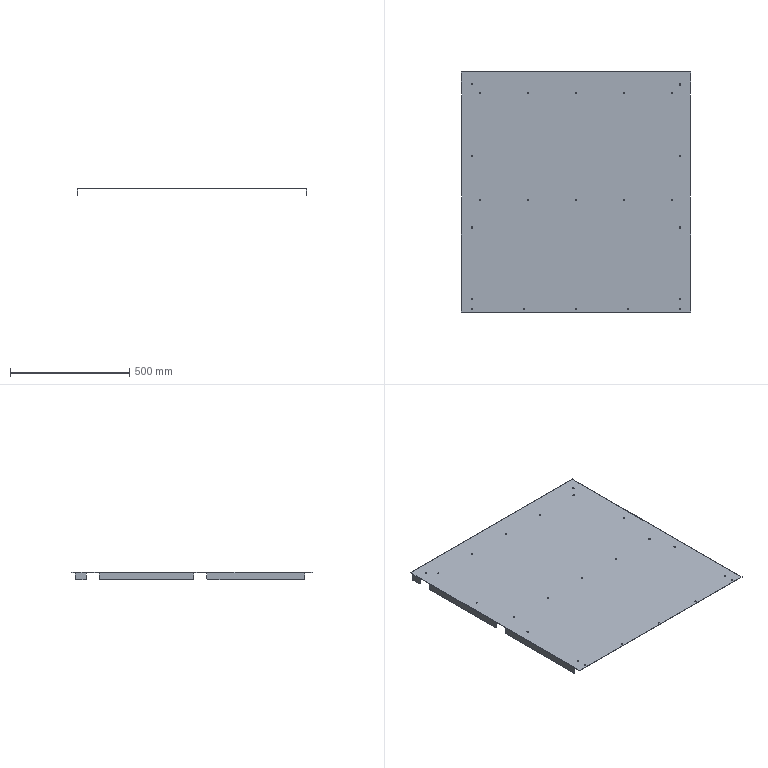Part | STEP file | SX-S19 | 1 solid | 124 faces | box 961 x 1005 x 30 mm | volume 1216636 mm3 | cylinder 70 | plane 54 | commonest cylinder face diameters 5.4 x42 10 x12 0.4 x6 2.8 x6 6.4 x4